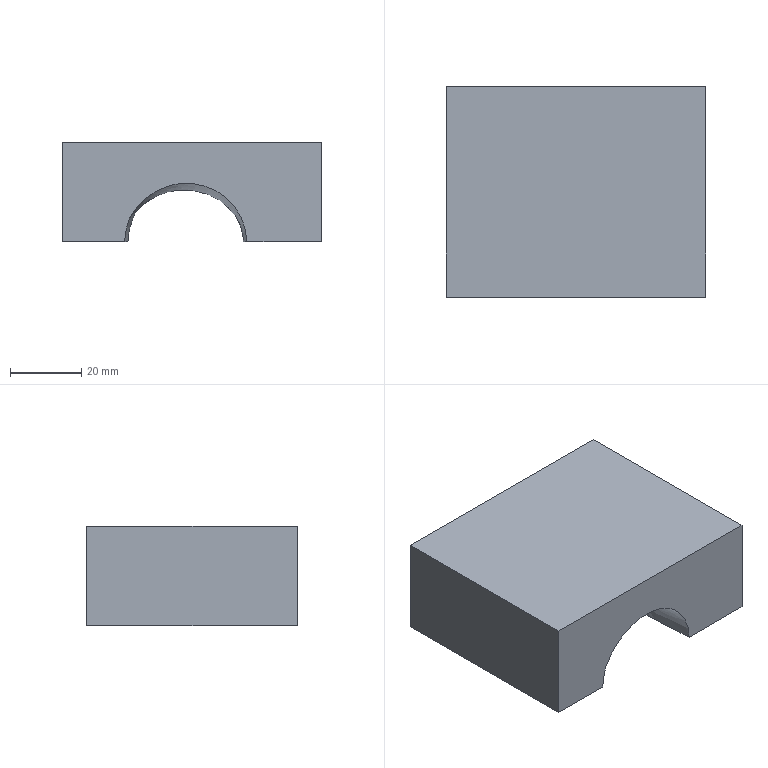NC program | NX | posted with a generic post | part box 72.744 x 59.015 x 27.972 mm
Whole program:
N10 G17 G21 G94 G90
(FLOOR_WALL , TOOL : D63)
N12 T03 M6
N14 G54
N16 G17 G0 G90 X-73.872 Y0. S6500 M3
N18 G43 Z30. H3
N20 Z3.
N22 G94 G1 Z0. F1500.
N24 X-70.872
N26 X70.872
N28 X73.872
N30 Z3.
N32 G0 Z30.
N34 M5
(ADAPTIVE_MILLING , TOOL : D10)
N36 T04 M6
N38 G54
N40 G17 G0 G90 X-47.091 Y0.033 S9500 M3
N42 G43 Z30. H4
N44 Z-10.986
N46 G94 G1 Z-13.986 F1000.
N48 X-46.251 Y-0.206 F3000.
N50 X-45.404 Y-0.421
N52 G3 X-44.444 Y0.033 R1.021
N54 X-43.751 Y2.421 R6.067
N56 X-43.405 Y10.059 R67.293
N58 G1 X-43.397 Y11.333
N60 X-43.39 Y12.983
N62 X-43.385 Y15.308
N64 X-43.382 Y19.208
N66 X-43.38 Y29.483
N68 X-43.377 Y29.633
N70 G2 X-40.945 Y33.847 R5.734
N72 X-35.326 Y35.985 R12.315
N74 X-26.346 Y36.466 R66.394
N76 G1 X-25.071 Y36.475
N78 X-23.496 Y36.482
N80 X-21.396 Y36.487
N82 X-17.946 Y36.491
N84 X-9.396 Y36.492
N86 X36.354
N88 G2 X40.635 Y34.198 R5.588
N90 X42.8 Y28.83 R11.712
N92 X43.315 Y20.979 R53.508
N94 G1 X43.326 Y20.08
N96 X43.336 Y18.955
N98 X43.344 Y17.53
N100 X43.35 Y15.655
N102 X43.355 Y12.955
N104 X43.357 Y8.005
N106 X43.358 Y-29.495
N108 X43.355 Y-29.645
N110 X43.352 Y-29.72
N112 X43.341 Y-29.87
N114 X43.334 Y-29.945
N116 G2 X40.424 Y-34.201 R6.085
N118 X34.772 Y-36.061 R13.513
N120 X25.787 Y-36.471 R77.312
N122 G1 X24.437 Y-36.479
N124 X22.637 Y-36.485
N126 X20.012 Y-36.49
N128 X15.287 Y-36.492
N130 X-21.163 Y-36.493
N132 X-36.388
N134 G2 X-40.691 Y-34.089 R5.671
N136 X-42.808 Y-28.698 R12.022
N138 X-43.324 Y-20.172 R58.445
N140 X-43.335 Y-2.997 R862.971
N142 X-42.711 Y3.12 R745.901
N144 G3 X-42.403 Y15.339 R181.731
N146 G1 X-42.397 Y17.739
N148 X-42.394 Y21.414
N150 X-42.392 Y26.439
N152 X-42.39 Y26.589
N154 X-42.384 Y26.738
N156 X-42.376 Y26.888
N158 X-42.372 Y26.956
N160 Y29.477
N162 X-42.368 Y29.537
N164 G2 X-40.062 Y34.23 R6.23
N166 X-36.342 Y35.507 R6.482
N168 G1 X36.342
N170 X36.401 Y35.504
N172 G2 X41.095 Y33.197 R6.23
N174 X42.372 Y29.477 R6.482
N176 G1 Y-29.477
N178 X42.368 Y-29.537
N180 G2 X40.062 Y-34.23 R6.23
N182 X36.342 Y-35.507 R6.482
N184 G1 X-36.342
N186 X-36.401 Y-35.504
N188 G2 X-41.095 Y-33.197 R6.23
N190 X-42.372 Y-29.477 R6.482
N192 G1 Y26.998
N194 G3 X-42.754 Y27.789 R1.026
N196 G1 X-44.872 Y29.47
N198 Z-10.986
N200 G0 Z30.
N202 X-47.093 Y0.031
N204 Z-24.972
N206 G1 Z-27.972 F1000.
N208 X-46.252 Y-0.208 F3000.
N210 X-45.406 Y-0.423
N212 G3 X-44.446 Y0.031 R1.021
N214 X-43.753 Y2.419 R6.067
N216 X-43.407 Y10.057 R67.293
N218 G1 X-43.399 Y11.332
N220 X-43.392 Y12.982
N222 X-43.387 Y15.307
N224 X-43.383 Y19.207
N226 X-43.382 Y29.482
N228 X-43.379 Y29.632
N230 G2 X-40.918 Y33.905 R5.705
N232 X-35.211 Y36.02 R12.423
N234 X-26.904 Y36.464 R65.406
N236 G1 X-25.779 Y36.473
N238 X-24.429 Y36.481
N240 X-22.554 Y36.487
N242 X-19.854 Y36.492
N244 X-14.604 Y36.494
N246 X36.396
N248 G2 X40.661 Y34.169 R5.61
N250 X42.83 Y28.643 R11.914
N252 X43.324 Y20.34 R59.242
N254 G1 X43.335 Y19.29
N256 X43.343 Y18.015
N258 X43.35 Y16.365
N260 X43.355 Y14.04
N262 X43.358 Y10.14
N264 X43.359 Y-2.91
N266 Y-29.535
N268 X43.358 Y-29.61
N270 X43.351 Y-29.76
N272 X43.346 Y-29.834
N274 G2 X40.644 Y-34.056 R5.945
N276 X35.109 Y-36.017 R12.864
N278 X26.502 Y-36.466 R67.472
N280 G1 X25.302 Y-36.476
N282 X23.727 Y-36.484
N284 X21.702 Y-36.489
N286 X18.552 Y-36.493
N288 X11.427 Y-36.495
N290 X-36.348
N292 G2 X-40.621 Y-34.182 R5.626
N294 X-42.816 Y-28.666 R11.935
N296 X-43.326 Y-20.139 R59.144
N298 G1 X-43.336 Y-19.014
N300 X-43.345 Y-17.664
N302 X-43.351 Y-15.939
N304 X-43.356 Y-13.464
N306 X-43.359 Y-9.039
N308 Y-3.714
N310 X-43.356 Y-3.489
N312 X-43.352 Y-3.339
N314 X-43.343 Y-3.115
N316 X-43.339 Y-3.04
N318 G2 X-42.728 Y2.928 R659.118
N320 G3 X-42.405 Y15.446 R177.202
N322 G1 X-42.399 Y17.921
N324 X-42.395 Y21.746
N326 X-42.394 Y26.396
N328 X-42.393 Y26.546
N330 X-42.389 Y26.696
N332 X-42.382 Y26.846
N334 X-42.372 Y27.009
N336 Y29.477
N338 X-42.368 Y29.537
N340 G2 X-40.062 Y34.23 R6.23
N342 X-36.342 Y35.507 R6.482
N344 G1 X36.342
N346 X36.401 Y35.504
N348 G2 X41.095 Y33.197 R6.23
N350 X42.372 Y29.477 R6.482
N352 G1 Y-29.477
N354 X42.368 Y-29.537
N356 G2 X40.062 Y-34.23 R6.23
N358 X36.342 Y-35.507 R6.482
N360 G1 X-36.342
N362 X-36.401 Y-35.504
N364 G2 X-41.095 Y-33.197 R6.23
N366 X-42.372 Y-29.477 R6.482
N368 G1 Y27.073
N370 G3 X-42.772 Y27.878 R1.025
N372 G1 X-44.872 Y29.47
N374 Z-24.972
N376 G0 Z30.
N378 M5
(ZLEVEL_PROFILE_COPY_COPY , TOOL : D10JING)
N380 T14 M6
N382 G54
N384 G17 G0 G90 X-37.468 Y35.406 S9500 M3
N386 G43 Z30. H14
N388 Z-13.986
N390 G94 G1 X-37.238 Y35.007 F1000.
N392 G3 X-36.372 Y34.507 R1.
N394 G1 X36.372 F1200.
N396 G2 X41.372 Y29.507 R5.
N398 G1 Y-29.507
N400 G2 X36.372 Y-34.507 R5.
N402 G1 X-36.372
N404 G2 X-41.372 Y-29.507 R5.
N406 G1 Y29.507
N408 G2 X-36.372 Y34.507 R5.
N410 G3 X-35.506 Y35.007 R1.
N412 G1 X-35.217 Y35.507
N414 G0 X-37.468 Y35.406 Z-27.972
N416 G1 X-37.238 Y35.007 F1000.
N418 G3 X-36.372 Y34.507 R1.
N420 G1 X36.372 F1200.
N422 G2 X41.372 Y29.507 R5.
N424 G1 Y-29.507
N426 G2 X36.372 Y-34.507 R5.
N428 G1 X-36.372
N430 G2 X-41.372 Y-29.507 R5.
N432 G1 Y29.507
N434 G2 X-36.372 Y34.507 R5.
N436 G3 X-35.506 Y35.007 R1.
N438 G1 X-35.217 Y35.507
N440 G0 Z30.
N442 M5
(ZLEVEL_PROFILE_1 , TOOL : D6A45)
N444 T01 M6
N446 G54
N448 G17 G0 G90 X-1.039 Y31.666 S9500 M3
N450 G43 Z30. H1
N452 Z0.5
N454 G94 G1 Z-1. F1250.
N456 X-0.52 Y30.766
N458 G3 X0. Y30.466 R0.6
N460 G1 X36.374
N462 G2 X37.33 Y29.518 R0.952
N464 G1 Y-29.51
N466 G2 X36.374 Y-30.466 R0.979
N468 G1 X-36.374
N470 G2 X-37.33 Y-29.51 R0.979
N472 G1 Y29.518
N474 G2 X-36.374 Y30.466 R0.952
N476 G1 X0.
N478 G3 X0.52 Y30.766 R0.6
N480 G1 X1.039 Y31.666
N482 Z0.5
N484 G0 Z30.
N486 M5
N488 M2